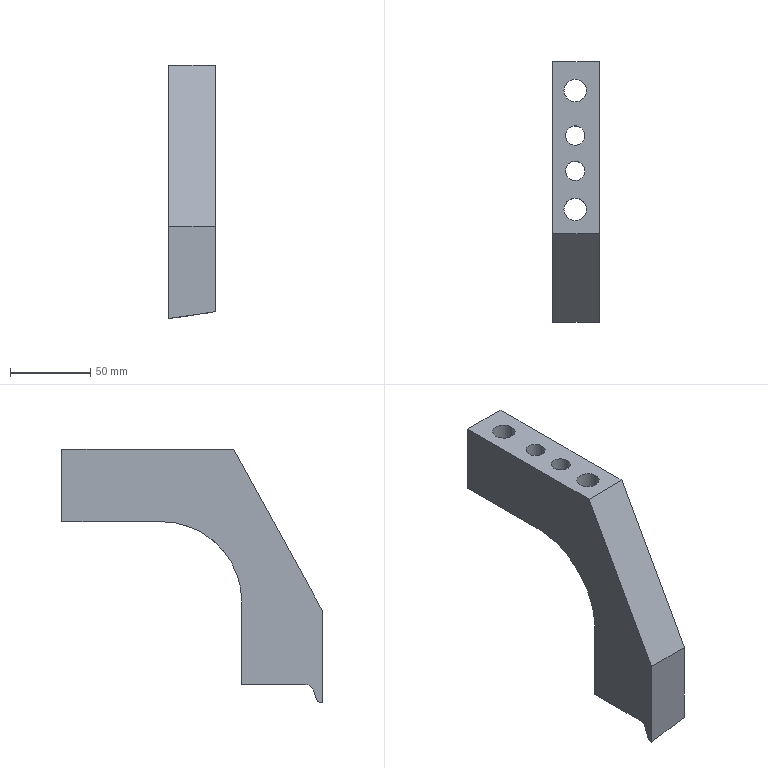Part | NX | features solid 2 | 1 solid | 24 faces | box 29 x 162 x 157.604 mm | volume 258550 mm3 | plane 10 | cylinder 7 | spline 7 | commonest cylinder face diameters 12 x2 14 x2 20 x2 100 x1
STEP:
#1=CARTESIAN_POINT('',(580.,-328.,55.));
#2=VERTEX_POINT('',#1);
#3=CARTESIAN_POINT('',(590.,-328.,55.));
#4=DIRECTION('',(0.,0.,-1.));
#5=DIRECTION('',(-1.,0.,0.));
#6=AXIS2_PLACEMENT_3D('',#3,#4,#5);
#7=CIRCLE('',#6,10.);
#8=EDGE_CURVE('',#2,#2,#7,.F.);
#9=ORIENTED_EDGE('',*,*,#8,.T.);
#10=EDGE_LOOP('',(#9));
#11=FACE_BOUND('',#10,.T.);
#12=CARTESIAN_POINT('',(584.,-356.,55.));
#13=VERTEX_POINT('',#12);
#14=CARTESIAN_POINT('',(590.,-356.,55.));
#15=DIRECTION('',(0.,0.,-1.));
#16=DIRECTION('',(-1.,0.,0.));
#17=AXIS2_PLACEMENT_3D('',#14,#15,#16);
#18=CIRCLE('',#17,6.);
#19=EDGE_CURVE('',#13,#13,#18,.T.);
#20=ORIENTED_EDGE('',*,*,#19,.F.);
#21=EDGE_LOOP('',(#20));
#22=FACE_BOUND('',#21,.T.);
#23=CARTESIAN_POINT('',(605.,-372.,55.));
#24=VERTEX_POINT('',#23);
#25=CARTESIAN_POINT('',(605.,-310.,55.));
#26=VERTEX_POINT('',#25);
#27=CARTESIAN_POINT('',(605.,-454.337,55.));
#28=DIRECTION('',(0.,1.,0.));
#29=VECTOR('',#28,1000.);
#30=LINE('',#27,#29);
#31=EDGE_CURVE('',#24,#26,#30,.T.);
#32=ORIENTED_EDGE('',*,*,#31,.F.);
#33=CARTESIAN_POINT('',(590.,-372.,55.));
#34=VERTEX_POINT('',#33);
#35=CARTESIAN_POINT('',(605.,-372.,55.));
#36=DIRECTION('',(-1.,0.,0.));
#37=VECTOR('',#36,1000.);
#38=LINE('',#35,#37);
#39=EDGE_CURVE('',#24,#34,#38,.T.);
#40=ORIENTED_EDGE('',*,*,#39,.T.);
#41=CARTESIAN_POINT('',(576.,-372.,55.));
#42=VERTEX_POINT('',#41);
#43=CARTESIAN_POINT('',(605.,-372.,55.));
#44=DIRECTION('',(-1.,0.,0.));
#45=VECTOR('',#44,1000.);
#46=LINE('',#43,#45);
#47=EDGE_CURVE('',#34,#42,#46,.T.);
#48=ORIENTED_EDGE('',*,*,#47,.T.);
#49=CARTESIAN_POINT('',(576.,-310.,55.));
#50=VERTEX_POINT('',#49);
#51=CARTESIAN_POINT('',(576.,-415.,55.));
#52=DIRECTION('',(0.,1.,0.));
#53=VECTOR('',#52,1000.);
#54=LINE('',#51,#53);
#55=EDGE_CURVE('',#42,#50,#54,.T.);
#56=ORIENTED_EDGE('',*,*,#55,.T.);
#57=CARTESIAN_POINT('',(605.,-310.,55.));
#58=DIRECTION('',(-1.,0.,0.));
#59=VECTOR('',#58,1000.);
#60=LINE('',#57,#59);
#61=EDGE_CURVE('',#26,#50,#60,.T.);
#62=ORIENTED_EDGE('',*,*,#61,.F.);
#63=EDGE_LOOP('',(#32,#40,#48,#56,#62));
#64=FACE_BOUND('',#63,.T.);
#65=CARTESIAN_POINT('',(605.,-415.,55.));
#66=DIRECTION('',(0.,0.,-1.));
#67=DIRECTION('',(-1.,0.,0.));
#68=AXIS2_PLACEMENT_3D('',#65,#66,#67);
#69=PLANE('',#68);
#70=ADVANCED_FACE('',(#11,#22,#64),#69,.T.);
#71=CARTESIAN_POINT('',(605.,-417.,100.));
#72=VERTEX_POINT('',#71);
#73=CARTESIAN_POINT('',(605.,-310.,100.));
#74=VERTEX_POINT('',#73);
#75=CARTESIAN_POINT('',(605.,-454.337,100.));
#76=DIRECTION('',(0.,-1.,0.));
#77=VECTOR('',#76,1000.);
#78=LINE('',#75,#77);
#79=EDGE_CURVE('',#72,#74,#78,.F.);
#80=ORIENTED_EDGE('',*,*,#79,.F.);
#81=CARTESIAN_POINT('',(605.,-472.,0.));
#82=VERTEX_POINT('',#81);
#83=CARTESIAN_POINT('',(605.,-552.351,-146.093));
#84=DIRECTION('',(0.,-0.4819,-0.8762));
#85=VECTOR('',#84,1000.);
#86=LINE('',#83,#85);
#87=EDGE_CURVE('',#72,#82,#86,.T.);
#88=ORIENTED_EDGE('',*,*,#87,.T.);
#89=CARTESIAN_POINT('',(605.,-472.,-53.264));
#90=VERTEX_POINT('',#89);
#91=CARTESIAN_POINT('',(605.,-472.,-200.));
#92=DIRECTION('',(0.,0.,1.));
#93=VECTOR('',#92,1000.);
#94=LINE('',#91,#93);
#95=EDGE_CURVE('',#90,#82,#94,.T.);
#96=ORIENTED_EDGE('',*,*,#95,.F.);
#97=CARTESIAN_POINT('',(605.,-471.443,-53.26));
#98=VERTEX_POINT('',#97);
#99=CARTESIAN_POINT('',(605.,-472.,-53.264));
#100=CARTESIAN_POINT('',(605.,-471.814,-53.263));
#101=CARTESIAN_POINT('',(605.,-471.629,-53.261));
#102=CARTESIAN_POINT('',(605.,-471.443,-53.26));
#103=B_SPLINE_CURVE_WITH_KNOTS('',3,(#99,#100,#101,#102),.UNSPECIFIED.,.F.,.F.,(4,4),(0.,0.0005568),.UNSPECIFIED.);
#104=EDGE_CURVE('',#90,#98,#103,.T.);
#105=ORIENTED_EDGE('',*,*,#104,.T.);
#106=CARTESIAN_POINT('',(605.,-468.638,-51.233));
#107=VERTEX_POINT('',#106);
#108=CARTESIAN_POINT('',(605.,-471.443,-53.26));
#109=CARTESIAN_POINT('',(605.,-470.204,-53.25));
#110=CARTESIAN_POINT('',(605.,-469.049,-52.404));
#111=CARTESIAN_POINT('',(605.,-468.639,-51.235));
#112=B_SPLINE_CURVE_WITH_KNOTS('',3,(#108,#109,#110,#111),.UNSPECIFIED.,.F.,.F.,(4,4),(0.,0.003664),.UNSPECIFIED.);
#113=EDGE_CURVE('',#98,#107,#112,.T.);
#114=ORIENTED_EDGE('',*,*,#113,.T.);
#115=CARTESIAN_POINT('',(605.,-466.595,-45.397));
#116=VERTEX_POINT('',#115);
#117=CARTESIAN_POINT('',(605.,-468.638,-51.233));
#118=CARTESIAN_POINT('',(605.,-467.957,-49.287));
#119=CARTESIAN_POINT('',(605.,-467.275,-47.341));
#120=CARTESIAN_POINT('',(605.,-466.594,-45.396));
#121=B_SPLINE_CURVE_WITH_KNOTS('',3,(#117,#118,#119,#120),.UNSPECIFIED.,.F.,.F.,(4,4),(0.0002323,0.006417),.UNSPECIFIED.);
#122=EDGE_CURVE('',#107,#116,#121,.T.);
#123=ORIENTED_EDGE('',*,*,#122,.T.);
#124=CARTESIAN_POINT('',(605.,-461.922,-42.022));
#125=VERTEX_POINT('',#124);
#126=CARTESIAN_POINT('',(605.,-466.595,-45.397));
#127=CARTESIAN_POINT('',(605.,-465.912,-43.449));
#128=CARTESIAN_POINT('',(605.,-463.987,-42.038));
#129=CARTESIAN_POINT('',(605.,-461.922,-42.022));
#130=B_SPLINE_CURVE_WITH_KNOTS('',3,(#126,#127,#128,#129),.UNSPECIFIED.,.F.,.F.,(4,4),(0.,0.006108),.UNSPECIFIED.);
#131=EDGE_CURVE('',#116,#125,#130,.T.);
#132=ORIENTED_EDGE('',*,*,#131,.T.);
#133=CARTESIAN_POINT('',(605.,-454.811,-41.967));
#134=VERTEX_POINT('',#133);
#135=CARTESIAN_POINT('',(605.,-461.922,-42.022));
#136=CARTESIAN_POINT('',(605.,-459.551,-42.003));
#137=CARTESIAN_POINT('',(605.,-457.181,-41.985));
#138=CARTESIAN_POINT('',(605.,-454.811,-41.967));
#139=B_SPLINE_CURVE_WITH_KNOTS('',3,(#135,#136,#137,#138),.UNSPECIFIED.,.F.,.F.,(4,4),(0.,0.007111),.UNSPECIFIED.);
#140=EDGE_CURVE('',#125,#134,#139,.T.);
#141=ORIENTED_EDGE('',*,*,#140,.T.);
#142=CARTESIAN_POINT('',(605.,-450.991,-40.891));
#143=VERTEX_POINT('',#142);
#144=CARTESIAN_POINT('',(605.,-454.811,-41.967));
#145=CARTESIAN_POINT('',(605.,-453.467,-41.956));
#146=CARTESIAN_POINT('',(605.,-452.132,-41.607));
#147=CARTESIAN_POINT('',(605.,-450.992,-40.892));
#148=B_SPLINE_CURVE_WITH_KNOTS('',3,(#144,#145,#146,#147),.UNSPECIFIED.,.F.,.F.,(4,4),(0.,0.004022),.UNSPECIFIED.);
#149=EDGE_CURVE('',#134,#143,#148,.T.);
#150=ORIENTED_EDGE('',*,*,#149,.T.);
#151=CARTESIAN_POINT('',(605.,-426.226,-40.665));
#152=VERTEX_POINT('',#151);
#153=CARTESIAN_POINT('',(605.,-426.227,-40.664));
#154=CARTESIAN_POINT('',(605.,-428.117,-39.5));
#155=CARTESIAN_POINT('',(605.,-432.05,-37.374));
#156=CARTESIAN_POINT('',(605.,-438.638,-35.963));
#157=CARTESIAN_POINT('',(605.,-445.204,-37.545));
#158=CARTESIAN_POINT('',(605.,-449.108,-39.71));
#159=CARTESIAN_POINT('',(605.,-450.99,-40.891));
#160=B_SPLINE_CURVE_WITH_KNOTS('',3,(#153,#154,#155,#156,#157,#158,#159),.UNSPECIFIED.,.F.,.F.,(4,1,1,1,4),(0.002201,0.008862,0.01552,0.02218,0.02885),.UNSPECIFIED.);
#161=EDGE_CURVE('',#152,#143,#160,.T.);
#162=ORIENTED_EDGE('',*,*,#161,.F.);
#163=CARTESIAN_POINT('',(605.,-422.331,-41.708));
#164=VERTEX_POINT('',#163);
#165=CARTESIAN_POINT('',(605.,-426.225,-40.666));
#166=CARTESIAN_POINT('',(605.,-425.061,-41.382));
#167=CARTESIAN_POINT('',(605.,-423.697,-41.719));
#168=CARTESIAN_POINT('',(605.,-422.331,-41.708));
#169=B_SPLINE_CURVE_WITH_KNOTS('',3,(#165,#166,#167,#168),.UNSPECIFIED.,.F.,.F.,(4,4),(0.,0.004086),.UNSPECIFIED.);
#170=EDGE_CURVE('',#152,#164,#169,.T.);
#171=ORIENTED_EDGE('',*,*,#170,.T.);
#172=CARTESIAN_POINT('',(605.,-422.,-41.706));
#173=VERTEX_POINT('',#172);
#174=CARTESIAN_POINT('',(605.,-422.331,-41.708));
#175=CARTESIAN_POINT('',(605.,-422.221,-41.708));
#176=CARTESIAN_POINT('',(605.,-422.11,-41.707));
#177=CARTESIAN_POINT('',(605.,-422.,-41.706));
#178=B_SPLINE_CURVE_WITH_KNOTS('',3,(#174,#175,#176,#177),.UNSPECIFIED.,.F.,.F.,(4,4),(0.03959,0.03992),.UNSPECIFIED.);
#179=EDGE_CURVE('',#164,#173,#178,.T.);
#180=ORIENTED_EDGE('',*,*,#179,.T.);
#181=CARTESIAN_POINT('',(605.,-422.,5.));
#182=VERTEX_POINT('',#181);
#183=CARTESIAN_POINT('',(605.,-422.,100.));
#184=DIRECTION('',(0.,0.,1.));
#185=VECTOR('',#184,1000.);
#186=LINE('',#183,#185);
#187=EDGE_CURVE('',#182,#173,#186,.F.);
#188=ORIENTED_EDGE('',*,*,#187,.F.);
#189=CARTESIAN_POINT('',(605.,-372.,5.));
#190=DIRECTION('',(1.,0.,0.));
#191=DIRECTION('',(0.,0.,-1.));
#192=AXIS2_PLACEMENT_3D('',#189,#190,#191);
#193=CIRCLE('',#192,50.);
#194=EDGE_CURVE('',#182,#24,#193,.F.);
#195=ORIENTED_EDGE('',*,*,#194,.T.);
#196=ORIENTED_EDGE('',*,*,#31,.T.);
#197=CARTESIAN_POINT('',(605.,-310.,-200.));
#198=DIRECTION('',(0.,0.,1.));
#199=VECTOR('',#198,1000.);
#200=LINE('',#197,#199);
#201=EDGE_CURVE('',#26,#74,#200,.T.);
#202=ORIENTED_EDGE('',*,*,#201,.T.);
#203=EDGE_LOOP('',(#80,#88,#96,#105,#114,#123,#132,#141,#150,#162,#171,#180,#188,#195,#196,#202));
#204=FACE_BOUND('',#203,.T.);
#205=CARTESIAN_POINT('',(605.,-454.337,-200.));
#206=DIRECTION('',(1.,0.,0.));
#207=DIRECTION('',(0.,0.,-1.));
#208=AXIS2_PLACEMENT_3D('',#205,#206,#207);
#209=PLANE('',#208);
#210=ADVANCED_FACE('',(#204),#209,.T.);
#211=ORIENTED_EDGE('',*,*,#95,.T.);
#212=CARTESIAN_POINT('',(576.,-472.,0.));
#213=VERTEX_POINT('',#212);
#214=CARTESIAN_POINT('',(590.5,-472.,0.));
#215=DIRECTION('',(-1.,0.,0.));
#216=VECTOR('',#215,1000.);
#217=LINE('',#214,#216);
#218=EDGE_CURVE('',#82,#213,#217,.T.);
#219=ORIENTED_EDGE('',*,*,#218,.T.);
#220=CARTESIAN_POINT('',(576.,-472.,-57.604));
#221=VERTEX_POINT('',#220);
#222=CARTESIAN_POINT('',(576.,-472.,-200.));
#223=DIRECTION('',(0.,0.,1.));
#224=VECTOR('',#223,1000.);
#225=LINE('',#222,#224);
#226=EDGE_CURVE('',#221,#213,#225,.T.);
#227=ORIENTED_EDGE('',*,*,#226,.F.);
#228=CARTESIAN_POINT('',(576.,-472.,-57.604));
#229=CARTESIAN_POINT('',(585.698,-472.,-56.366));
#230=CARTESIAN_POINT('',(595.365,-472.,-54.919));
#231=CARTESIAN_POINT('',(605.,-472.,-53.264));
#232=B_SPLINE_CURVE_WITH_KNOTS('',3,(#228,#229,#230,#231),.UNSPECIFIED.,.F.,.F.,(4,4),(0.,0.02932),.UNSPECIFIED.);
#233=EDGE_CURVE('',#221,#90,#232,.T.);
#234=ORIENTED_EDGE('',*,*,#233,.T.);
#235=EDGE_LOOP('',(#211,#219,#227,#234));
#236=FACE_BOUND('',#235,.T.);
#237=CARTESIAN_POINT('',(590.5,-472.,80.));
#238=DIRECTION('',(0.,1.,0.));
#239=DIRECTION('',(0.,0.,1.));
#240=AXIS2_PLACEMENT_3D('',#237,#238,#239);
#241=PLANE('',#240);
#242=ADVANCED_FACE('',(#236),#241,.F.);
#243=ORIENTED_EDGE('',*,*,#226,.T.);
#244=CARTESIAN_POINT('',(576.,-417.,100.));
#245=VERTEX_POINT('',#244);
#246=CARTESIAN_POINT('',(576.,-417.,100.));
#247=DIRECTION('',(0.,0.4819,0.8762));
#248=VECTOR('',#247,1000.);
#249=LINE('',#246,#248);
#250=EDGE_CURVE('',#213,#245,#249,.T.);
#251=ORIENTED_EDGE('',*,*,#250,.T.);
#252=CARTESIAN_POINT('',(576.,-310.,100.));
#253=VERTEX_POINT('',#252);
#254=CARTESIAN_POINT('',(576.,-454.412,100.));
#255=DIRECTION('',(0.,-1.,0.));
#256=VECTOR('',#255,1000.);
#257=LINE('',#254,#256);
#258=EDGE_CURVE('',#245,#253,#257,.F.);
#259=ORIENTED_EDGE('',*,*,#258,.T.);
#260=CARTESIAN_POINT('',(576.,-310.,-200.));
#261=DIRECTION('',(0.,0.,1.));
#262=VECTOR('',#261,1000.);
#263=LINE('',#260,#262);
#264=EDGE_CURVE('',#50,#253,#263,.T.);
#265=ORIENTED_EDGE('',*,*,#264,.F.);
#266=ORIENTED_EDGE('',*,*,#55,.F.);
#267=CARTESIAN_POINT('',(576.,-422.,5.));
#268=VERTEX_POINT('',#267);
#269=CARTESIAN_POINT('',(576.,-372.,5.));
#270=DIRECTION('',(1.,0.,0.));
#271=DIRECTION('',(0.,0.,-1.));
#272=AXIS2_PLACEMENT_3D('',#269,#270,#271);
#273=CIRCLE('',#272,50.);
#274=EDGE_CURVE('',#42,#268,#273,.T.);
#275=ORIENTED_EDGE('',*,*,#274,.T.);
#276=CARTESIAN_POINT('',(576.,-422.,-46.119));
#277=VERTEX_POINT('',#276);
#278=CARTESIAN_POINT('',(576.,-422.,100.));
#279=DIRECTION('',(0.,0.,-1.));
#280=VECTOR('',#279,1000.);
#281=LINE('',#278,#280);
#282=EDGE_CURVE('',#268,#277,#281,.T.);
#283=ORIENTED_EDGE('',*,*,#282,.T.);
#284=CARTESIAN_POINT('',(576.,-461.922,-46.435));
#285=VERTEX_POINT('',#284);
#286=CARTESIAN_POINT('',(576.,-422.,-46.119));
#287=CARTESIAN_POINT('',(576.,-435.307,-46.227));
#288=CARTESIAN_POINT('',(576.,-448.615,-46.332));
#289=CARTESIAN_POINT('',(576.,-461.922,-46.435));
#290=B_SPLINE_CURVE_WITH_KNOTS('',3,(#286,#287,#288,#289),.UNSPECIFIED.,.F.,.F.,(4,4),(0.,0.03992),.UNSPECIFIED.);
#291=EDGE_CURVE('',#277,#285,#290,.T.);
#292=ORIENTED_EDGE('',*,*,#291,.T.);
#293=CARTESIAN_POINT('',(576.,-466.595,-49.789));
#294=VERTEX_POINT('',#293);
#295=CARTESIAN_POINT('',(576.,-461.922,-46.435));
#296=CARTESIAN_POINT('',(576.,-463.982,-46.451));
#297=CARTESIAN_POINT('',(576.,-465.911,-47.846));
#298=CARTESIAN_POINT('',(576.,-466.595,-49.789));
#299=B_SPLINE_CURVE_WITH_KNOTS('',3,(#295,#296,#297,#298),.UNSPECIFIED.,.F.,.F.,(4,4),(0.,0.006092),.UNSPECIFIED.);
#300=EDGE_CURVE('',#285,#294,#299,.T.);
#301=ORIENTED_EDGE('',*,*,#300,.T.);
#302=CARTESIAN_POINT('',(576.,-468.639,-55.588));
#303=VERTEX_POINT('',#302);
#304=CARTESIAN_POINT('',(576.,-466.595,-49.789));
#305=CARTESIAN_POINT('',(576.,-467.276,-51.722));
#306=CARTESIAN_POINT('',(576.,-467.957,-53.655));
#307=CARTESIAN_POINT('',(576.,-468.639,-55.588));
#308=B_SPLINE_CURVE_WITH_KNOTS('',3,(#304,#305,#306,#307),.UNSPECIFIED.,.F.,.F.,(4,4),(0.001441,0.00759),.UNSPECIFIED.);
#309=EDGE_CURVE('',#294,#303,#308,.T.);
#310=ORIENTED_EDGE('',*,*,#309,.T.);
#311=CARTESIAN_POINT('',(576.,-471.443,-57.6));
#312=VERTEX_POINT('',#311);
#313=CARTESIAN_POINT('',(576.,-468.639,-55.588));
#314=CARTESIAN_POINT('',(576.,-469.05,-56.754));
#315=CARTESIAN_POINT('',(576.,-470.207,-57.591));
#316=CARTESIAN_POINT('',(576.,-471.443,-57.6));
#317=B_SPLINE_CURVE_WITH_KNOTS('',3,(#313,#314,#315,#316),.UNSPECIFIED.,.F.,.F.,(4,4),(0.,0.003655),.UNSPECIFIED.);
#318=EDGE_CURVE('',#303,#312,#317,.T.);
#319=ORIENTED_EDGE('',*,*,#318,.T.);
#320=CARTESIAN_POINT('',(576.,-471.443,-57.6));
#321=CARTESIAN_POINT('',(576.,-471.629,-57.602));
#322=CARTESIAN_POINT('',(576.,-471.814,-57.603));
#323=CARTESIAN_POINT('',(576.,-472.,-57.604));
#324=B_SPLINE_CURVE_WITH_KNOTS('',3,(#320,#321,#322,#323),.UNSPECIFIED.,.F.,.F.,(4,4),(0.04944,0.05),.UNSPECIFIED.);
#325=EDGE_CURVE('',#312,#221,#324,.T.);
#326=ORIENTED_EDGE('',*,*,#325,.T.);
#327=EDGE_LOOP('',(#243,#251,#259,#265,#266,#275,#283,#292,#301,#310,#319,#326));
#328=FACE_BOUND('',#327,.T.);
#329=CARTESIAN_POINT('',(576.,-454.412,-200.));
#330=DIRECTION('',(1.,0.,0.));
#331=DIRECTION('',(0.,0.,-1.));
#332=AXIS2_PLACEMENT_3D('',#329,#330,#331);
#333=PLANE('',#332);
#334=ADVANCED_FACE('',(#328),#333,.F.);
#335=CARTESIAN_POINT('',(597.,-328.,75.));
#336=VERTEX_POINT('',#335);
#337=CARTESIAN_POINT('',(590.,-328.,75.));
#338=DIRECTION('',(0.,0.,1.));
#339=DIRECTION('',(1.,0.,0.));
#340=AXIS2_PLACEMENT_3D('',#337,#338,#339);
#341=CIRCLE('',#340,7.);
#342=EDGE_CURVE('',#336,#336,#341,.T.);
#343=ORIENTED_EDGE('',*,*,#342,.F.);
#344=EDGE_LOOP('',(#343));
#345=FACE_BOUND('',#344,.T.);
#346=CARTESIAN_POINT('',(597.,-328.,100.));
#347=VERTEX_POINT('',#346);
#348=CARTESIAN_POINT('',(590.,-328.,100.));
#349=DIRECTION('',(0.,0.,1.));
#350=DIRECTION('',(1.,0.,0.));
#351=AXIS2_PLACEMENT_3D('',#348,#349,#350);
#352=CIRCLE('',#351,7.);
#353=EDGE_CURVE('',#347,#347,#352,.F.);
#354=ORIENTED_EDGE('',*,*,#353,.F.);
#355=EDGE_LOOP('',(#354));
#356=FACE_BOUND('',#355,.T.);
#357=CARTESIAN_POINT('',(590.,-328.,75.));
#358=DIRECTION('',(0.,0.,1.));
#359=DIRECTION('',(-1.,0.,0.));
#360=AXIS2_PLACEMENT_3D('',#357,#358,#359);
#361=CYLINDRICAL_SURFACE('',#360,7.);
#362=ADVANCED_FACE('',(#345,#356),#361,.F.);
#363=CARTESIAN_POINT('',(597.,-402.,75.));
#364=VERTEX_POINT('',#363);
#365=CARTESIAN_POINT('',(590.,-402.,75.));
#366=DIRECTION('',(0.,0.,1.));
#367=DIRECTION('',(1.,0.,0.));
#368=AXIS2_PLACEMENT_3D('',#365,#366,#367);
#369=CIRCLE('',#368,7.);
#370=EDGE_CURVE('',#364,#364,#369,.T.);
#371=ORIENTED_EDGE('',*,*,#370,.F.);
#372=EDGE_LOOP('',(#371));
#373=FACE_BOUND('',#372,.T.);
#374=CARTESIAN_POINT('',(597.,-402.,100.));
#375=VERTEX_POINT('',#374);
#376=CARTESIAN_POINT('',(590.,-402.,100.));
#377=DIRECTION('',(0.,0.,1.));
#378=DIRECTION('',(1.,0.,0.));
#379=AXIS2_PLACEMENT_3D('',#376,#377,#378);
#380=CIRCLE('',#379,7.);
#381=EDGE_CURVE('',#375,#375,#380,.F.);
#382=ORIENTED_EDGE('',*,*,#381,.F.);
#383=EDGE_LOOP('',(#382));
#384=FACE_BOUND('',#383,.T.);
#385=CARTESIAN_POINT('',(590.,-402.,75.));
#386=DIRECTION('',(0.,0.,1.));
#387=DIRECTION('',(-1.,0.,0.));
#388=AXIS2_PLACEMENT_3D('',#385,#386,#387);
#389=CYLINDRICAL_SURFACE('',#388,7.);
#390=ADVANCED_FACE('',(#373,#384),#389,.F.);
#391=ORIENTED_EDGE('',*,*,#342,.T.);
#392=EDGE_LOOP('',(#391));
#393=FACE_BOUND('',#392,.T.);
#394=CARTESIAN_POINT('',(600.,-328.,75.));
#395=VERTEX_POINT('',#394);
#396=CARTESIAN_POINT('',(590.,-328.,75.));
#397=DIRECTION('',(0.,0.,-1.));
#398=DIRECTION('',(1.,0.,0.));
#399=AXIS2_PLACEMENT_3D('',#396,#397,#398);
#400=CIRCLE('',#399,10.);
#401=EDGE_CURVE('',#395,#395,#400,.T.);
#402=ORIENTED_EDGE('',*,*,#401,.T.);
#403=EDGE_LOOP('',(#402));
#404=FACE_BOUND('',#403,.T.);
#405=CARTESIAN_POINT('',(590.,-328.,75.));
#406=DIRECTION('',(0.,0.,1.));
#407=DIRECTION('',(-1.,0.,0.));
#408=AXIS2_PLACEMENT_3D('',#405,#406,#407);
#409=PLANE('',#408);
#410=ADVANCED_FACE('',(#393,#404),#409,.F.);
#411=ORIENTED_EDGE('',*,*,#370,.T.);
#412=EDGE_LOOP('',(#411));
#413=FACE_BOUND('',#412,.T.);
#414=CARTESIAN_POINT('',(600.,-402.,75.));
#415=VERTEX_POINT('',#414);
#416=CARTESIAN_POINT('',(590.,-402.,75.));
#417=DIRECTION('',(0.,0.,-1.));
#418=DIRECTION('',(1.,0.,0.));
#419=AXIS2_PLACEMENT_3D('',#416,#417,#418);
#420=CIRCLE('',#419,10.);
#421=EDGE_CURVE('',#415,#415,#420,.T.);
#422=ORIENTED_EDGE('',*,*,#421,.T.);
#423=EDGE_LOOP('',(#422));
#424=FACE_BOUND('',#423,.T.);
#425=CARTESIAN_POINT('',(590.,-402.,75.));
#426=DIRECTION('',(0.,0.,1.));
#427=DIRECTION('',(-1.,0.,0.));
#428=AXIS2_PLACEMENT_3D('',#425,#426,#427);
#429=PLANE('',#428);
#430=ADVANCED_FACE('',(#413,#424),#429,.F.);
#431=ORIENTED_EDGE('',*,*,#258,.F.);
#432=CARTESIAN_POINT('',(675.,-417.,100.));
#433=DIRECTION('',(-1.,0.,0.));
#434=VECTOR('',#433,1000.);
#435=LINE('',#432,#434);
#436=EDGE_CURVE('',#245,#72,#435,.F.);
#437=ORIENTED_EDGE('',*,*,#436,.T.);
#438=ORIENTED_EDGE('',*,*,#79,.T.);
#439=CARTESIAN_POINT('',(650.,-310.,100.));
#440=DIRECTION('',(1.,0.,0.));
#441=VECTOR('',#440,1000.);
#442=LINE('',#439,#441);
#443=EDGE_CURVE('',#74,#253,#442,.F.);
#444=ORIENTED_EDGE('',*,*,#443,.T.);
#445=EDGE_LOOP('',(#431,#437,#438,#444));
#446=FACE_BOUND('',#445,.T.);
#447=ORIENTED_EDGE('',*,*,#353,.T.);
#448=EDGE_LOOP('',(#447));
#449=FACE_BOUND('',#448,.T.);
#450=ORIENTED_EDGE('',*,*,#381,.T.);
#451=EDGE_LOOP('',(#450));
#452=FACE_BOUND('',#451,.T.);
#453=CARTESIAN_POINT('',(596.,-356.,100.));
#454=VERTEX_POINT('',#453);
#455=CARTESIAN_POINT('',(590.,-356.,100.));
#456=DIRECTION('',(0.,0.,1.));
#457=DIRECTION('',(1.,0.,0.));
#458=AXIS2_PLACEMENT_3D('',#455,#456,#457);
#459=CIRCLE('',#458,6.);
#460=EDGE_CURVE('',#454,#454,#459,.F.);
#461=ORIENTED_EDGE('',*,*,#460,.T.);
#462=EDGE_LOOP('',(#461));
#463=FACE_BOUND('',#462,.T.);
#464=CARTESIAN_POINT('',(596.,-378.,100.));
#465=VERTEX_POINT('',#464);
#466=CARTESIAN_POINT('',(590.,-378.,100.));
#467=DIRECTION('',(0.,0.,1.));
#468=DIRECTION('',(1.,0.,0.));
#469=AXIS2_PLACEMENT_3D('',#466,#467,#468);
#470=CIRCLE('',#469,6.);
#471=EDGE_CURVE('',#465,#465,#470,.F.);
#472=ORIENTED_EDGE('',*,*,#471,.T.);
#473=EDGE_LOOP('',(#472));
#474=FACE_BOUND('',#473,.T.);
#475=CARTESIAN_POINT('',(675.,-230.,100.));
#476=DIRECTION('',(0.,0.,1.));
#477=DIRECTION('',(-1.,0.,0.));
#478=AXIS2_PLACEMENT_3D('',#475,#476,#477);
#479=PLANE('',#478);
#480=ADVANCED_FACE('',(#446,#449,#452,#463,#474),#479,.T.);
#481=ORIENTED_EDGE('',*,*,#401,.F.);
#482=EDGE_LOOP('',(#481));
#483=FACE_BOUND('',#482,.T.);
#484=ORIENTED_EDGE('',*,*,#8,.F.);
#485=EDGE_LOOP('',(#484));
#486=FACE_BOUND('',#485,.T.);
#487=CARTESIAN_POINT('',(590.,-328.,75.));
#488=DIRECTION('',(0.,0.,-1.));
#489=DIRECTION('',(1.,0.,0.));
#490=AXIS2_PLACEMENT_3D('',#487,#488,#489);
#491=CYLINDRICAL_SURFACE('',#490,10.);
#492=ADVANCED_FACE('',(#483,#486),#491,.F.);
#493=ORIENTED_EDGE('',*,*,#201,.F.);
#494=ORIENTED_EDGE('',*,*,#61,.T.);
#495=ORIENTED_EDGE('',*,*,#264,.T.);
#496=ORIENTED_EDGE('',*,*,#443,.F.);
#497=EDGE_LOOP('',(#493,#494,#495,#496));
#498=FACE_BOUND('',#497,.T.);
#499=CARTESIAN_POINT('',(650.,-310.,75.));
#500=DIRECTION('',(0.,1.,0.));
#501=DIRECTION('',(0.,0.,1.));
#502=AXIS2_PLACEMENT_3D('',#499,#500,#501);
#503=PLANE('',#502);
#504=ADVANCED_FACE('',(#498),#503,.T.);
#505=ORIENTED_EDGE('',*,*,#421,.F.);
#506=EDGE_LOOP('',(#505));
#507=FACE_BOUND('',#506,.T.);
#508=CARTESIAN_POINT('',(599.148,-397.961,47.732));
#509=VERTEX_POINT('',#508);
#510=CARTESIAN_POINT('',(600.213,-401.668,45.333));
#511=CARTESIAN_POINT('',(599.412,-397.91,47.836));
#512=CARTESIAN_POINT('',(597.025,-394.457,49.714));
#513=CARTESIAN_POINT('',(593.167,-392.157,50.763));
#514=CARTESIAN_POINT('',(588.548,-391.754,50.931));
#515=CARTESIAN_POINT('',(584.265,-393.414,50.209));
#516=CARTESIAN_POINT('',(581.284,-396.55,48.621));
#517=CARTESIAN_POINT('',(579.913,-400.276,46.32));
#518=CARTESIAN_POINT('',(579.978,-403.91,43.581));
#519=CARTESIAN_POINT('',(581.205,-407.146,40.645));
#520=CARTESIAN_POINT('',(583.415,-409.806,37.789));
#521=CARTESIAN_POINT('',(586.238,-411.458,35.723));
#522=CARTESIAN_POINT('',(589.141,-412.05,34.933));
#523=CARTESIAN_POINT('',(591.43,-411.983,35.024));
#524=CARTESIAN_POINT('',(593.543,-411.428,35.755));
#525=CARTESIAN_POINT('',(595.895,-410.25,37.231));
#526=CARTESIAN_POINT('',(598.089,-408.209,39.559));
#527=CARTESIAN_POINT('',(599.694,-405.156,42.511));
#528=CARTESIAN_POINT('',(600.213,-401.668,45.333));
#529=CARTESIAN_POINT('',(599.412,-397.91,47.836));
#530=CARTESIAN_POINT('',(597.025,-394.457,49.714));
#531=B_SPLINE_CURVE_WITH_KNOTS('',3,(#510,#511,#512,#513,#514,#515,#516,#517,#518,#519,#520,#521,#522,#523,#524,#525,#526,#527,#528,#529,#530),.UNSPECIFIED.,.T.,.F.,(1,1,1,1,1,1,1,1,1,1,1,1,1,1,1,1,1,1,1,1,1,1,1,1,1),(-0.01343,-0.008956,-0.004478,0.,0.004478,0.008956,0.01343,0.01791,0.02239,0.02687,0.03135,0.03582,0.0403,0.04478,0.04702,0.04926,0.0515,0.05374,0.05822,0.06269,0.06717,0.07165,0.07613,0.08061,0.08508),.UNSPECIFIED.);
#532=EDGE_CURVE('',#509,#509,#531,.T.);
#533=ORIENTED_EDGE('',*,*,#532,.F.);
#534=EDGE_LOOP('',(#533));
#535=FACE_BOUND('',#534,.T.);
#536=CARTESIAN_POINT('',(590.,-402.,75.));
#537=DIRECTION('',(0.,0.,-1.));
#538=DIRECTION('',(1.,0.,0.));
#539=AXIS2_PLACEMENT_3D('',#536,#537,#538);
#540=CYLINDRICAL_SURFACE('',#539,10.);
#541=ADVANCED_FACE('',(#507,#535),#540,.F.);
#542=ORIENTED_EDGE('',*,*,#460,.F.);
#543=EDGE_LOOP('',(#542));
#544=FACE_BOUND('',#543,.T.);
#545=ORIENTED_EDGE('',*,*,#19,.T.);
#546=EDGE_LOOP('',(#545));
#547=FACE_BOUND('',#546,.T.);
#548=CARTESIAN_POINT('',(590.,-356.,105.));
#549=DIRECTION('',(0.,0.,-1.));
#550=DIRECTION('',(-1.,0.,0.));
#551=AXIS2_PLACEMENT_3D('',#548,#549,#550);
#552=CYLINDRICAL_SURFACE('',#551,6.);
#553=ADVANCED_FACE('',(#544,#547),#552,.F.);
#554=ORIENTED_EDGE('',*,*,#471,.F.);
#555=EDGE_LOOP('',(#554));
#556=FACE_BOUND('',#555,.T.);
#557=CARTESIAN_POINT('',(585.273,-373.312,55.025));
#558=CARTESIAN_POINT('',(590.001,-371.345,54.988));
#559=CARTESIAN_POINT('',(594.722,-373.308,55.025));
#560=CARTESIAN_POINT('',(596.643,-378.043,54.725));
#561=CARTESIAN_POINT('',(594.706,-382.687,53.888));
#562=CARTESIAN_POINT('',(589.997,-384.657,53.364));
#563=CARTESIAN_POINT('',(585.294,-382.685,53.888));
#564=CARTESIAN_POINT('',(583.359,-378.047,54.724));
#565=CARTESIAN_POINT('',(585.273,-373.312,55.025));
#566=CARTESIAN_POINT('',(590.001,-371.345,54.988));
#567=CARTESIAN_POINT('',(594.722,-373.308,55.025));
#568=B_SPLINE_CURVE_WITH_KNOTS('',3,(#557,#558,#559,#560,#561,#562,#563,#564,#565,#566,#567),.UNSPECIFIED.,.T.,.F.,(1,1,1,1,1,1,1,1,1,1,1,1,1,1,1),(0.004713,0.009424,0.01414,0.01885,0.02356,0.02827,0.03298,0.03769,0.0424,0.04711,0.05182,0.05654,0.06125,0.06596,0.07067),.UNSPECIFIED.);
#569=EDGE_CURVE('',#34,#34,#568,.T.);
#570=ORIENTED_EDGE('',*,*,#569,.T.);
#571=EDGE_LOOP('',(#570));
#572=FACE_BOUND('',#571,.T.);
#573=CARTESIAN_POINT('',(590.,-378.,105.));
#574=DIRECTION('',(0.,0.,-1.));
#575=DIRECTION('',(-1.,0.,0.));
#576=AXIS2_PLACEMENT_3D('',#573,#574,#575);
#577=CYLINDRICAL_SURFACE('',#576,6.);
#578=ADVANCED_FACE('',(#556,#572),#577,.F.);
#579=ORIENTED_EDGE('',*,*,#282,.F.);
#580=CARTESIAN_POINT('',(576.,-422.,5.));
#581=DIRECTION('',(-1.,0.,0.));
#582=VECTOR('',#581,1000.);
#583=LINE('',#580,#582);
#584=EDGE_CURVE('',#268,#182,#583,.F.);
#585=ORIENTED_EDGE('',*,*,#584,.T.);
#586=ORIENTED_EDGE('',*,*,#187,.T.);
#587=CARTESIAN_POINT('',(605.,-422.,-41.706));
#588=CARTESIAN_POINT('',(595.366,-422.,-43.389));
#589=CARTESIAN_POINT('',(585.699,-422.,-44.86));
#590=CARTESIAN_POINT('',(576.,-422.,-46.119));
#591=B_SPLINE_CURVE_WITH_KNOTS('',3,(#587,#588,#589,#590),.UNSPECIFIED.,.F.,.F.,(4,4),(0.,0.02933),.UNSPECIFIED.);
#592=EDGE_CURVE('',#173,#277,#591,.T.);
#593=ORIENTED_EDGE('',*,*,#592,.T.);
#594=EDGE_LOOP('',(#579,#585,#586,#593));
#595=FACE_BOUND('',#594,.T.);
#596=CARTESIAN_POINT('',(576.,-422.,100.));
#597=DIRECTION('',(0.,-1.,0.));
#598=DIRECTION('',(1.,0.,0.));
#599=AXIS2_PLACEMENT_3D('',#596,#597,#598);
#600=PLANE('',#599);
#601=ADVANCED_FACE('',(#595),#600,.F.);
#602=CARTESIAN_POINT('',(605.,-450.992,-40.892));
#603=CARTESIAN_POINT('',(603.356,-449.446,-41.202));
#604=CARTESIAN_POINT('',(600.638,-445.621,-41.683));
#605=CARTESIAN_POINT('',(599.169,-438.575,-41.888));
#606=CARTESIAN_POINT('',(600.665,-431.558,-41.551));
#607=CARTESIAN_POINT('',(603.37,-427.762,-41.002));
#608=CARTESIAN_POINT('',(605.,-426.225,-40.666));
#609=B_SPLINE_CURVE_WITH_KNOTS('',3,(#602,#603,#604,#605,#606,#607,#608),.UNSPECIFIED.,.F.,.F.,(4,1,1,1,4),(0.2827,0.3907,0.4987,0.6067,0.7147),.UNSPECIFIED.);
#610=EDGE_CURVE('',#143,#152,#609,.T.);
#611=ORIENTED_EDGE('',*,*,#610,.F.);
#612=ORIENTED_EDGE('',*,*,#149,.F.);
#613=CARTESIAN_POINT('',(605.,-422.331,-41.708));
#614=CARTESIAN_POINT('',(602.584,-424.169,-42.145));
#615=CARTESIAN_POINT('',(598.483,-429.013,-42.872));
#616=CARTESIAN_POINT('',(596.16,-438.527,-43.321));
#617=CARTESIAN_POINT('',(598.441,-448.084,-43.031));
#618=CARTESIAN_POINT('',(602.565,-452.966,-42.377));
#619=CARTESIAN_POINT('',(605.,-454.811,-41.967));
#620=B_SPLINE_CURVE_WITH_KNOTS('',3,(#613,#614,#615,#616,#617,#618,#619),.UNSPECIFIED.,.F.,.F.,(4,1,1,1,4),(0.2502,0.3755,0.5009,0.6262,0.7515),.UNSPECIFIED.);
#621=EDGE_CURVE('',#164,#134,#620,.T.);
#622=ORIENTED_EDGE('',*,*,#621,.F.);
#623=ORIENTED_EDGE('',*,*,#170,.F.);
#624=EDGE_LOOP('',(#611,#612,#622,#623));
#625=FACE_BOUND('',#624,.T.);
#626=CARTESIAN_POINT('',(606.794,-452.461,-40.547));
#627=CARTESIAN_POINT('',(606.559,-452.879,-41.01));
#628=CARTESIAN_POINT('',(606.27,-453.354,-41.394));
#629=CARTESIAN_POINT('',(605.934,-453.87,-41.683));
#630=CARTESIAN_POINT('',(605.565,-454.406,-41.865));
#631=CARTESIAN_POINT('',(605.176,-454.943,-41.937));
#632=CARTESIAN_POINT('',(606.572,-452.303,-40.591));
#633=CARTESIAN_POINT('',(606.331,-452.717,-41.053));
#634=CARTESIAN_POINT('',(606.034,-453.185,-41.436));
#635=CARTESIAN_POINT('',(605.691,-453.693,-41.725));
#636=CARTESIAN_POINT('',(605.314,-454.222,-41.907));
#637=CARTESIAN_POINT('',(604.918,-454.751,-41.98));
#638=CARTESIAN_POINT('',(606.353,-452.141,-40.633));
#639=CARTESIAN_POINT('',(606.105,-452.549,-41.094));
#640=CARTESIAN_POINT('',(605.801,-453.011,-41.478));
#641=CARTESIAN_POINT('',(605.451,-453.512,-41.766));
#642=CARTESIAN_POINT('',(605.066,-454.033,-41.949));
#643=CARTESIAN_POINT('',(604.663,-454.554,-42.023));
#644=CARTESIAN_POINT('',(606.136,-451.974,-40.675));
#645=CARTESIAN_POINT('',(605.882,-452.376,-41.135));
#646=CARTESIAN_POINT('',(605.572,-452.832,-41.518));
#647=CARTESIAN_POINT('',(605.214,-453.325,-41.807));
#648=CARTESIAN_POINT('',(604.822,-453.838,-41.99));
#649=CARTESIAN_POINT('',(604.412,-454.352,-42.066));
#650=CARTESIAN_POINT('',(603.575,-449.911,-41.168));
#651=CARTESIAN_POINT('',(603.244,-450.245,-41.619));
#652=CARTESIAN_POINT('',(602.852,-450.62,-41.997));
#653=CARTESIAN_POINT('',(602.408,-451.024,-42.285));
#654=CARTESIAN_POINT('',(601.931,-451.443,-42.475));
#655=CARTESIAN_POINT('',(601.436,-451.863,-42.562));
#656=CARTESIAN_POINT('',(601.472,-447.185,-41.543));
#657=CARTESIAN_POINT('',(601.081,-447.433,-41.988));
#658=CARTESIAN_POINT('',(600.625,-447.712,-42.363));
#659=CARTESIAN_POINT('',(600.116,-448.011,-42.652));
#660=CARTESIAN_POINT('',(599.572,-448.321,-42.846));
#661=CARTESIAN_POINT('',(599.012,-448.631,-42.941));
#662=CARTESIAN_POINT('',(600.129,-444.211,-41.763));
#663=CARTESIAN_POINT('',(599.701,-444.372,-42.204));
#664=CARTESIAN_POINT('',(599.206,-444.551,-42.577));
#665=CARTESIAN_POINT('',(598.656,-444.744,-42.866));
#666=CARTESIAN_POINT('',(598.071,-444.945,-43.062));
#667=CARTESIAN_POINT('',(597.471,-445.146,-43.162));
#668=CARTESIAN_POINT('',(599.007,-438.121,-41.915));
#669=CARTESIAN_POINT('',(598.547,-438.104,-42.355));
#670=CARTESIAN_POINT('',(598.017,-438.086,-42.727));
#671=CARTESIAN_POINT('',(597.432,-438.068,-43.016));
#672=CARTESIAN_POINT('',(596.811,-438.051,-43.214));
#673=CARTESIAN_POINT('',(596.175,-438.034,-43.316));
#674=CARTESIAN_POINT('',(600.528,-432.181,-41.58));
#675=CARTESIAN_POINT('',(600.11,-431.99,-42.026));
#676=CARTESIAN_POINT('',(599.623,-431.777,-42.4));
#677=CARTESIAN_POINT('',(599.081,-431.55,-42.69));
#678=CARTESIAN_POINT('',(598.504,-431.316,-42.884));
#679=CARTESIAN_POINT('',(597.91,-431.083,-42.979));
#680=CARTESIAN_POINT('',(601.839,-429.583,-41.314));
#681=CARTESIAN_POINT('',(601.457,-429.313,-41.763));
#682=CARTESIAN_POINT('',(601.007,-429.012,-42.141));
#683=CARTESIAN_POINT('',(600.504,-428.69,-42.43));
#684=CARTESIAN_POINT('',(599.965,-428.358,-42.621));
#685=CARTESIAN_POINT('',(599.41,-428.026,-42.711));
#686=CARTESIAN_POINT('',(603.792,-427.139,-40.917));
#687=CARTESIAN_POINT('',(603.465,-426.792,-41.374));
#688=CARTESIAN_POINT('',(603.075,-426.403,-41.755));
#689=CARTESIAN_POINT('',(602.632,-425.984,-42.044));
#690=CARTESIAN_POINT('',(602.154,-425.55,-42.23));
#691=CARTESIAN_POINT('',(601.657,-425.118,-42.311));
#692=CARTESIAN_POINT('',(606.127,-425.247,-40.432));
#693=CARTESIAN_POINT('',(605.87,-424.836,-40.898));
#694=CARTESIAN_POINT('',(605.554,-424.372,-41.285));
#695=CARTESIAN_POINT('',(605.188,-423.869,-41.574));
#696=CARTESIAN_POINT('',(604.788,-423.347,-41.754));
#697=CARTESIAN_POINT('',(604.368,-422.827,-41.823));
#698=CARTESIAN_POINT('',(606.355,-425.07,-40.385));
#699=CARTESIAN_POINT('',(606.105,-424.653,-40.852));
#700=CARTESIAN_POINT('',(605.796,-424.182,-41.239));
#701=CARTESIAN_POINT('',(605.438,-423.671,-41.528));
#702=CARTESIAN_POINT('',(605.045,-423.141,-41.707));
#703=CARTESIAN_POINT('',(604.633,-422.612,-41.775));
#704=CARTESIAN_POINT('',(606.586,-424.898,-40.336));
#705=CARTESIAN_POINT('',(606.343,-424.476,-40.805));
#706=CARTESIAN_POINT('',(606.042,-423.997,-41.192));
#707=CARTESIAN_POINT('',(605.692,-423.479,-41.481));
#708=CARTESIAN_POINT('',(605.307,-422.94,-41.66));
#709=CARTESIAN_POINT('',(604.902,-422.403,-41.726));
#710=CARTESIAN_POINT('',(606.821,-424.732,-40.287));
#711=CARTESIAN_POINT('',(606.585,-424.304,-40.757));
#712=CARTESIAN_POINT('',(606.291,-423.818,-41.145));
#713=CARTESIAN_POINT('',(605.949,-423.292,-41.434));
#714=CARTESIAN_POINT('',(605.572,-422.746,-41.612));
#715=CARTESIAN_POINT('',(605.175,-422.2,-41.677));
#716=B_SPLINE_SURFACE_WITH_KNOTS('',5,5,((#626,#627,#628,#629,#630,#631),(#632,#633,#634,#635,#636,#637),(#638,#639,#640,#641,#642,#643),(#644,#645,#646,#647,#648,#649),(#650,#651,#652,#653,#654,#655),(#656,#657,#658,#659,#660,#661),(#662,#663,#664,#665,#666,#667),(#668,#669,#670,#671,#672,#673),(#674,#675,#676,#677,#678,#679),(#680,#681,#682,#683,#684,#685),(#686,#687,#688,#689,#690,#691),(#692,#693,#694,#695,#696,#697),(#698,#699,#700,#701,#702,#703),(#704,#705,#706,#707,#708,#709),(#710,#711,#712,#713,#714,#715)),.UNSPECIFIED.,.F.,.F.,.F.,(6,3,3,3,6),(6,6),(0.2455,0.2674,0.5097,0.7294,0.7528),(0.,1.),.UNSPECIFIED.);
#717=ADVANCED_FACE('',(#625),#716,.F.);
#718=ORIENTED_EDGE('',*,*,#161,.T.);
#719=ORIENTED_EDGE('',*,*,#610,.T.);
#720=EDGE_LOOP('',(#718,#719));
#721=FACE_BOUND('',#720,.T.);
#722=CARTESIAN_POINT('',(608.418,-428.741,-36.423));
#723=CARTESIAN_POINT('',(604.166,-425.36,-41.856));
#724=CARTESIAN_POINT('',(606.613,-431.011,-36.423));
#725=CARTESIAN_POINT('',(601.731,-428.423,-41.856));
#726=CARTESIAN_POINT('',(605.337,-433.702,-36.423));
#727=CARTESIAN_POINT('',(600.009,-432.053,-41.856));
#728=CARTESIAN_POINT('',(604.718,-436.651,-36.423));
#729=CARTESIAN_POINT('',(599.174,-436.031,-41.856));
#730=CARTESIAN_POINT('',(604.857,-440.997,-36.423));
#731=CARTESIAN_POINT('',(599.362,-441.894,-41.856));
#732=CARTESIAN_POINT('',(606.387,-444.97,-36.423));
#733=CARTESIAN_POINT('',(601.426,-447.255,-41.856));
#734=CARTESIAN_POINT('',(606.994,-446.154,-36.423));
#735=CARTESIAN_POINT('',(602.245,-448.852,-41.856));
#736=CARTESIAN_POINT('',(607.722,-447.264,-36.423));
#737=CARTESIAN_POINT('',(603.227,-450.349,-41.856));
#738=CARTESIAN_POINT('',(608.559,-448.286,-36.423));
#739=CARTESIAN_POINT('',(604.355,-451.727,-41.856));
#740=B_SPLINE_SURFACE_WITH_KNOTS('',5,1,((#722,#723),(#724,#725),(#726,#727),(#728,#729),(#730,#731),(#732,#733),(#734,#735),(#736,#737),(#738,#739)),.RULED_SURF.,.F.,.F.,.F.,(6,3,6),(2,2),(0.2864,0.5838,0.7186),(0.07273,1.),.UNSPECIFIED.);
#741=ADVANCED_FACE('',(#721),#740,.T.);
#742=ORIENTED_EDGE('',*,*,#233,.F.);
#743=ORIENTED_EDGE('',*,*,#325,.F.);
#744=CARTESIAN_POINT('',(576.,-471.443,-57.6));
#745=CARTESIAN_POINT('',(585.708,-471.443,-56.36));
#746=CARTESIAN_POINT('',(595.374,-471.443,-54.913));
#747=CARTESIAN_POINT('',(605.,-471.443,-53.26));
#748=B_SPLINE_CURVE_WITH_KNOTS('',3,(#744,#745,#746,#747),.UNSPECIFIED.,.F.,.F.,(4,4),(0.1181,0.4086),.UNSPECIFIED.);
#749=EDGE_CURVE('',#312,#98,#748,.T.);
#750=ORIENTED_EDGE('',*,*,#749,.T.);
#751=ORIENTED_EDGE('',*,*,#104,.F.);
#752=EDGE_LOOP('',(#742,#743,#750,#751));
#753=FACE_BOUND('',#752,.T.);
#754=CARTESIAN_POINT('',(575.825,-471.443,-57.623));
#755=CARTESIAN_POINT('',(575.825,-471.583,-57.624));
#756=CARTESIAN_POINT('',(575.825,-471.723,-57.625));
#757=CARTESIAN_POINT('',(575.825,-471.863,-57.626));
#758=CARTESIAN_POINT('',(575.825,-472.003,-57.627));
#759=CARTESIAN_POINT('',(581.72,-471.443,-56.871));
#760=CARTESIAN_POINT('',(581.72,-471.583,-56.872));
#761=CARTESIAN_POINT('',(581.72,-471.723,-56.873));
#762=CARTESIAN_POINT('',(581.72,-471.863,-56.874));
#763=CARTESIAN_POINT('',(581.72,-472.003,-56.875));
#764=CARTESIAN_POINT('',(587.602,-471.443,-56.056));
#765=CARTESIAN_POINT('',(587.602,-471.583,-56.057));
#766=CARTESIAN_POINT('',(587.602,-471.723,-56.058));
#767=CARTESIAN_POINT('',(587.602,-471.863,-56.059));
#768=CARTESIAN_POINT('',(587.602,-472.003,-56.06));
#769=CARTESIAN_POINT('',(593.472,-471.443,-55.178));
#770=CARTESIAN_POINT('',(593.472,-471.583,-55.179));
#771=CARTESIAN_POINT('',(593.472,-471.723,-55.18));
#772=CARTESIAN_POINT('',(593.472,-471.863,-55.181));
#773=CARTESIAN_POINT('',(593.472,-472.003,-55.182));
#774=CARTESIAN_POINT('',(599.329,-471.443,-54.236));
#775=CARTESIAN_POINT('',(599.329,-471.583,-54.237));
#776=CARTESIAN_POINT('',(599.329,-471.723,-54.238));
#777=CARTESIAN_POINT('',(599.329,-471.863,-54.239));
#778=CARTESIAN_POINT('',(599.329,-472.003,-54.24));
#779=CARTESIAN_POINT('',(605.173,-471.443,-53.23));
#780=CARTESIAN_POINT('',(605.173,-471.583,-53.231));
#781=CARTESIAN_POINT('',(605.173,-471.723,-53.232));
#782=CARTESIAN_POINT('',(605.173,-471.863,-53.233));
#783=CARTESIAN_POINT('',(605.173,-472.003,-53.234));
#784=B_SPLINE_SURFACE_WITH_KNOTS('',5,4,((#754,#755,#756,#757,#758),(#759,#760,#761,#762,#763),(#764,#765,#766,#767,#768),(#769,#770,#771,#772,#773),(#774,#775,#776,#777,#778),(#779,#780,#781,#782,#783)),.UNSPECIFIED.,.F.,.F.,.F.,(6,6),(5,5),(0.2266,0.415),(0.9846,0.9854),.PIECEWISE_BEZIER_KNOTS.);
#785=ADVANCED_FACE('',(#753),#784,.T.);
#786=ORIENTED_EDGE('',*,*,#749,.F.);
#787=ORIENTED_EDGE('',*,*,#318,.F.);
#788=CARTESIAN_POINT('',(576.,-468.639,-55.588));
#789=CARTESIAN_POINT('',(585.702,-468.639,-54.345));
#790=CARTESIAN_POINT('',(595.371,-468.639,-52.894));
#791=CARTESIAN_POINT('',(605.,-468.639,-51.235));
#792=B_SPLINE_CURVE_WITH_KNOTS('',3,(#788,#789,#790,#791),.UNSPECIFIED.,.F.,.F.,(4,4),(0.122,0.413),.UNSPECIFIED.);
#793=EDGE_CURVE('',#303,#107,#792,.T.);
#794=ORIENTED_EDGE('',*,*,#793,.T.);
#795=ORIENTED_EDGE('',*,*,#113,.F.);
#796=EDGE_LOOP('',(#786,#787,#794,#795));
#797=FACE_BOUND('',#796,.T.);
#798=CARTESIAN_POINT('',(605.514,-471.443,-53.171));
#799=CARTESIAN_POINT('',(605.513,-470.71,-53.166));
#800=CARTESIAN_POINT('',(605.474,-469.979,-52.939));
#801=CARTESIAN_POINT('',(605.397,-469.341,-52.492));
#802=CARTESIAN_POINT('',(605.292,-468.885,-51.885));
#803=CARTESIAN_POINT('',(605.175,-468.639,-51.205));
#804=CARTESIAN_POINT('',(599.599,-471.443,-54.192));
#805=CARTESIAN_POINT('',(599.598,-470.71,-54.186));
#806=CARTESIAN_POINT('',(599.561,-469.979,-53.96));
#807=CARTESIAN_POINT('',(599.488,-469.341,-53.512));
#808=CARTESIAN_POINT('',(599.389,-468.885,-52.904));
#809=CARTESIAN_POINT('',(599.277,-468.639,-52.223));
#810=CARTESIAN_POINT('',(593.672,-471.443,-55.147));
#811=CARTESIAN_POINT('',(593.671,-470.71,-55.142));
#812=CARTESIAN_POINT('',(593.636,-469.979,-54.915));
#813=CARTESIAN_POINT('',(593.567,-469.341,-54.467));
#814=CARTESIAN_POINT('',(593.473,-468.885,-53.858));
#815=CARTESIAN_POINT('',(593.368,-468.639,-53.175));
#816=CARTESIAN_POINT('',(587.734,-471.443,-56.038));
#817=CARTESIAN_POINT('',(587.733,-470.71,-56.032));
#818=CARTESIAN_POINT('',(587.7,-469.979,-55.805));
#819=CARTESIAN_POINT('',(587.634,-469.341,-55.356));
#820=CARTESIAN_POINT('',(587.546,-468.885,-54.747));
#821=CARTESIAN_POINT('',(587.446,-468.639,-54.063));
#822=CARTESIAN_POINT('',(581.784,-471.443,-56.863));
#823=CARTESIAN_POINT('',(581.783,-470.71,-56.857));
#824=CARTESIAN_POINT('',(581.752,-469.979,-56.63));
#825=CARTESIAN_POINT('',(581.691,-469.341,-56.18));
#826=CARTESIAN_POINT('',(581.607,-468.885,-55.57));
#827=CARTESIAN_POINT('',(581.514,-468.639,-54.886));
#828=CARTESIAN_POINT('',(575.823,-471.443,-57.623));
#829=CARTESIAN_POINT('',(575.823,-470.71,-57.617));
#830=CARTESIAN_POINT('',(575.794,-469.979,-57.389));
#831=CARTESIAN_POINT('',(575.736,-469.341,-56.939));
#832=CARTESIAN_POINT('',(575.658,-468.885,-56.328));
#833=CARTESIAN_POINT('',(575.571,-468.639,-55.643));
#834=B_SPLINE_SURFACE_WITH_KNOTS('',5,5,((#798,#799,#800,#801,#802,#803),(#804,#805,#806,#807,#808,#809),(#810,#811,#812,#813,#814,#815),(#816,#817,#818,#819,#820,#821),(#822,#823,#824,#825,#826,#827),(#828,#829,#830,#831,#832,#833)),.UNSPECIFIED.,.F.,.F.,.F.,(6,6),(6,6),(0.5852,0.8823),(0.,1.),.PIECEWISE_BEZIER_KNOTS.);
#835=ADVANCED_FACE('',(#797),#834,.T.);
#836=ORIENTED_EDGE('',*,*,#793,.F.);
#837=ORIENTED_EDGE('',*,*,#309,.F.);
#838=CARTESIAN_POINT('',(576.,-466.595,-49.789));
#839=CARTESIAN_POINT('',(585.83,-466.594,-48.518));
#840=CARTESIAN_POINT('',(595.501,-466.594,-47.047));
#841=CARTESIAN_POINT('',(605.,-466.594,-45.396));
#842=B_SPLINE_CURVE_WITH_KNOTS('',3,(#838,#839,#840,#841),.UNSPECIFIED.,.F.,.F.,(4,4),(0.1368,0.4468),.UNSPECIFIED.);
#843=EDGE_CURVE('',#294,#116,#842,.T.);
#844=ORIENTED_EDGE('',*,*,#843,.T.);
#845=ORIENTED_EDGE('',*,*,#122,.F.);
#846=EDGE_LOOP('',(#836,#837,#844,#845));
#847=FACE_BOUND('',#846,.T.);
#848=CARTESIAN_POINT('',(575.824,-468.651,-55.646));
#849=CARTESIAN_POINT('',(585.969,-468.661,-54.377));
#850=CARTESIAN_POINT('',(596.083,-468.673,-52.885));
#851=CARTESIAN_POINT('',(606.163,-468.686,-51.168));
#852=CARTESIAN_POINT('',(575.092,-466.547,-49.77));
#853=CARTESIAN_POINT('',(585.15,-466.557,-48.513));
#854=CARTESIAN_POINT('',(595.178,-466.569,-47.033));
#855=CARTESIAN_POINT('',(605.172,-466.582,-45.331));
#856=(BOUNDED_SURFACE()B_SPLINE_SURFACE(1,3,((#848,#849,#850,#851),(#852,#853,#854,#855)),.CONICAL_SURF.,.F.,.F.,.F.)B_SPLINE_SURFACE_WITH_KNOTS((2,2),(4,4),(0.1017,0.8469),(0.2619,0.5151),.PIECEWISE_BEZIER_KNOTS.)GEOMETRIC_REPRESENTATION_ITEM()RATIONAL_B_SPLINE_SURFACE(((0.9985,0.9982,0.9981,0.9981),(0.9985,0.9982,0.9981,0.9981)))REPRESENTATION_ITEM('')SURFACE());
#857=ADVANCED_FACE('',(#847),#856,.T.);
#858=ORIENTED_EDGE('',*,*,#843,.F.);
#859=ORIENTED_EDGE('',*,*,#300,.F.);
#860=CARTESIAN_POINT('',(605.,-461.922,-42.022));
#861=CARTESIAN_POINT('',(595.372,-461.922,-43.704));
#862=CARTESIAN_POINT('',(585.703,-461.922,-45.175));
#863=CARTESIAN_POINT('',(576.,-461.922,-46.435));
#864=B_SPLINE_CURVE_WITH_KNOTS('',3,(#860,#861,#862,#863),.UNSPECIFIED.,.F.,.F.,(4,4),(0.5356,0.8533),.UNSPECIFIED.);
#865=EDGE_CURVE('',#125,#285,#864,.T.);
#866=ORIENTED_EDGE('',*,*,#865,.F.);
#867=ORIENTED_EDGE('',*,*,#131,.F.);
#868=EDGE_LOOP('',(#858,#859,#866,#867));
#869=FACE_BOUND('',#868,.T.);
#870=CARTESIAN_POINT('',(575.822,-466.595,-49.812));
#871=CARTESIAN_POINT('',(575.675,-466.186,-48.67));
#872=CARTESIAN_POINT('',(575.543,-465.426,-47.652));
#873=CARTESIAN_POINT('',(575.447,-464.363,-46.902));
#874=CARTESIAN_POINT('',(575.398,-463.144,-46.523));
#875=CARTESIAN_POINT('',(575.396,-461.922,-46.514));
#876=CARTESIAN_POINT('',(581.831,-466.595,-49.037));
#877=CARTESIAN_POINT('',(581.673,-466.186,-47.897));
#878=CARTESIAN_POINT('',(581.533,-465.425,-46.88));
#879=CARTESIAN_POINT('',(581.429,-464.363,-46.131));
#880=CARTESIAN_POINT('',(581.377,-463.144,-45.752));
#881=CARTESIAN_POINT('',(581.376,-461.922,-45.742));
#882=CARTESIAN_POINT('',(587.828,-466.595,-48.195));
#883=CARTESIAN_POINT('',(587.66,-466.186,-47.056));
#884=CARTESIAN_POINT('',(587.511,-465.425,-46.041));
#885=CARTESIAN_POINT('',(587.401,-464.363,-45.292));
#886=CARTESIAN_POINT('',(587.345,-463.144,-44.914));
#887=CARTESIAN_POINT('',(587.344,-461.922,-44.905));
#888=CARTESIAN_POINT('',(593.814,-466.595,-47.286));
#889=CARTESIAN_POINT('',(593.636,-466.186,-46.149));
#890=CARTESIAN_POINT('',(593.477,-465.425,-45.135));
#891=CARTESIAN_POINT('',(593.36,-464.362,-44.387));
#892=CARTESIAN_POINT('',(593.301,-463.144,-44.01));
#893=CARTESIAN_POINT('',(593.3,-461.922,-44.));
#894=CARTESIAN_POINT('',(599.788,-466.595,-46.31));
#895=CARTESIAN_POINT('',(599.6,-466.186,-45.174));
#896=CARTESIAN_POINT('',(599.432,-465.425,-44.162));
#897=CARTESIAN_POINT('',(599.308,-464.362,-43.416));
#898=CARTESIAN_POINT('',(599.246,-463.143,-43.038));
#899=CARTESIAN_POINT('',(599.244,-461.922,-43.029));
#900=CARTESIAN_POINT('',(605.749,-466.595,-45.267));
#901=CARTESIAN_POINT('',(605.551,-466.186,-44.133));
#902=CARTESIAN_POINT('',(605.374,-465.425,-43.122));
#903=CARTESIAN_POINT('',(605.243,-464.362,-42.377));
#904=CARTESIAN_POINT('',(605.177,-463.143,-42.));
#905=CARTESIAN_POINT('',(605.176,-461.922,-41.991));
#906=B_SPLINE_SURFACE_WITH_KNOTS('',5,5,((#870,#871,#872,#873,#874,#875),(#876,#877,#878,#879,#880,#881),(#882,#883,#884,#885,#886,#887),(#888,#889,#890,#891,#892,#893),(#894,#895,#896,#897,#898,#899),(#900,#901,#902,#903,#904,#905)),.UNSPECIFIED.,.F.,.F.,.F.,(6,6),(6,6),(0.1401,0.4663),(0.,1.),.PIECEWISE_BEZIER_KNOTS.);
#907=ADVANCED_FACE('',(#869),#906,.F.);
#908=ORIENTED_EDGE('',*,*,#865,.T.);
#909=ORIENTED_EDGE('',*,*,#291,.F.);
#910=ORIENTED_EDGE('',*,*,#592,.F.);
#911=ORIENTED_EDGE('',*,*,#179,.F.);
#912=ORIENTED_EDGE('',*,*,#621,.T.);
#913=ORIENTED_EDGE('',*,*,#140,.F.);
#914=EDGE_LOOP('',(#908,#909,#910,#911,#912,#913));
#915=FACE_BOUND('',#914,.T.);
#916=CARTESIAN_POINT('',(575.808,-421.76,-46.142));
#917=CARTESIAN_POINT('',(575.814,-435.148,-46.25));
#918=CARTESIAN_POINT('',(575.82,-448.535,-46.355));
#919=CARTESIAN_POINT('',(575.825,-461.922,-46.458));
#920=CARTESIAN_POINT('',(581.707,-421.76,-45.378));
#921=CARTESIAN_POINT('',(581.713,-435.148,-45.485));
#922=CARTESIAN_POINT('',(581.718,-448.535,-45.591));
#923=CARTESIAN_POINT('',(581.723,-461.922,-45.694));
#924=CARTESIAN_POINT('',(587.593,-421.76,-44.549));
#925=CARTESIAN_POINT('',(587.598,-435.148,-44.656));
#926=CARTESIAN_POINT('',(587.603,-448.535,-44.761));
#927=CARTESIAN_POINT('',(587.608,-461.922,-44.865));
#928=CARTESIAN_POINT('',(593.466,-421.76,-43.655));
#929=CARTESIAN_POINT('',(593.471,-435.147,-43.762));
#930=CARTESIAN_POINT('',(593.476,-448.535,-43.868));
#931=CARTESIAN_POINT('',(593.48,-461.922,-43.971));
#932=CARTESIAN_POINT('',(599.326,-421.76,-42.697));
#933=CARTESIAN_POINT('',(599.331,-435.147,-42.804));
#934=CARTESIAN_POINT('',(599.335,-448.535,-42.909));
#935=CARTESIAN_POINT('',(599.34,-461.922,-43.012));
#936=CARTESIAN_POINT('',(605.173,-421.76,-41.674));
#937=CARTESIAN_POINT('',(605.178,-435.147,-41.781));
#938=CARTESIAN_POINT('',(605.182,-448.534,-41.886));
#939=CARTESIAN_POINT('',(605.186,-461.922,-41.989));
#940=B_SPLINE_SURFACE_WITH_KNOTS('',5,3,((#916,#917,#918,#919),(#920,#921,#922,#923),(#924,#925,#926,#927),(#928,#929,#930,#931),(#932,#933,#934,#935),(#936,#937,#938,#939)),.UNSPECIFIED.,.F.,.F.,.F.,(6,6),(4,4),(0.1482,0.4681),(0.8178,1.),.PIECEWISE_BEZIER_KNOTS.);
#941=ADVANCED_FACE('',(#915),#940,.T.);
#942=ORIENTED_EDGE('',*,*,#194,.F.);
#943=ORIENTED_EDGE('',*,*,#584,.F.);
#944=ORIENTED_EDGE('',*,*,#274,.F.);
#945=ORIENTED_EDGE('',*,*,#47,.F.);
#946=ORIENTED_EDGE('',*,*,#569,.F.);
#947=ORIENTED_EDGE('',*,*,#39,.F.);
#948=EDGE_LOOP('',(#942,#943,#944,#945,#946,#947));
#949=FACE_BOUND('',#948,.T.);
#950=ORIENTED_EDGE('',*,*,#532,.T.);
#951=EDGE_LOOP('',(#950));
#952=FACE_BOUND('',#951,.T.);
#953=CARTESIAN_POINT('',(605.,-372.,5.));
#954=DIRECTION('',(-1.,0.,0.));
#955=DIRECTION('',(0.,0.,1.));
#956=AXIS2_PLACEMENT_3D('',#953,#954,#955);
#957=CYLINDRICAL_SURFACE('',#956,50.);
#958=ADVANCED_FACE('',(#949,#952),#957,.F.);
#959=ORIENTED_EDGE('',*,*,#250,.F.);
#960=ORIENTED_EDGE('',*,*,#218,.F.);
#961=ORIENTED_EDGE('',*,*,#87,.F.);
#962=ORIENTED_EDGE('',*,*,#436,.F.);
#963=EDGE_LOOP('',(#959,#960,#961,#962));
#964=FACE_BOUND('',#963,.T.);
#965=CARTESIAN_POINT('',(675.,-417.,100.));
#966=DIRECTION('',(0.,-0.8762,0.4819));
#967=DIRECTION('',(0.,-0.4819,-0.8762));
#968=AXIS2_PLACEMENT_3D('',#965,#966,#967);
#969=PLANE('',#968);
#970=ADVANCED_FACE('',(#964),#969,.T.);
#971=CLOSED_SHELL('',(#70,#210,#242,#334,#362,#390,#410,#430,#480,#492,#504,#541,#553,#578,#601,#717,#741,#785,#835,#857,#907,#941,#958,#970));
#972=MANIFOLD_SOLID_BREP('',#971);
#973=(LENGTH_UNIT()NAMED_UNIT(*)SI_UNIT(.MILLI.,.METRE.));
#974=UNCERTAINTY_MEASURE_WITH_UNIT(LENGTH_MEASURE(0.05478),#973,'','');
#975=(NAMED_UNIT(*)PLANE_ANGLE_UNIT()SI_UNIT($,.RADIAN.));
#976=(NAMED_UNIT(*)SI_UNIT($,.STERADIAN.)SOLID_ANGLE_UNIT());
#977=(GEOMETRIC_REPRESENTATION_CONTEXT(3)GLOBAL_UNCERTAINTY_ASSIGNED_CONTEXT((#974))GLOBAL_UNIT_ASSIGNED_CONTEXT((#973,#975,#976))REPRESENTATION_CONTEXT('',''));
#978=ADVANCED_BREP_SHAPE_REPRESENTATION('',(#972),#977);